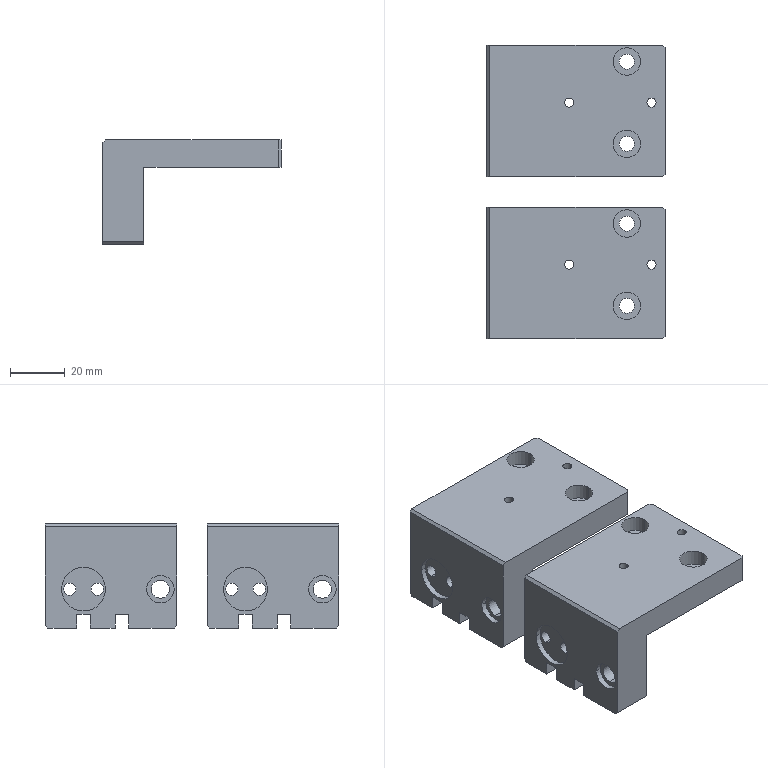NC program | NX | posted with a generic post | part box 65 x 107 x 38 mm
Whole program:
N10 G17 G21 G94 G90
(DRILLING_COPY , TOOL : D6A45)
N12 T01 M6
N14 G54
N16 G17 G0 G90 X-15. Y-4.8 B0. C0. S5000 M3
N18 G43 Z30. H1
N20 G94 G81 G98 Z-1. F350. R3.
N22 X-5.
N24 X18.
N26 G80
N28 G0 X18. Y-4.8 Z30.
N30 M5
(DRILLING_COPY_COPY_COPY_1 , TOOL : 4.5ZT)
N32 T08 M6
N34 G54
N36 G17 G0 G90 X-5. Y-4.8 B0. C0. S2000 M3
N38 G43 Z30. H8
N40 G94 G83 G98 Z-17.352 F300. Q2. R3.
N42 X-15.
N44 G80
N46 G0 X-15. Y-4.8 Z30.
N48 M5
(DRILLING_COPY_COPY_COPY_1_COPY , TOOL : 6.6ZT)
N50 T10 M6
N52 G54
N54 G17 G0 G90 X18. Y-4.8 B0. C0. S2000 M3
N56 G43 Z30. H10
N58 G94 G83 G98 Z-17.983 F300. Q2. R3.
N60 G80
N62 G0 X18. Y-4.8 Z30.
N64 M5
(HOLE_MILLING_COPY , TOOL : D6)
N66 T12 M6
N68 G54
N70 G17 G0 G90 X-10. Y-4.8 B0. C0. S9500 M3
N72 G43 Z30. H12
N74 Z0.5
N76 G94 G3 X-11.225 Y-3.575 R1.225 F1500.
N78 X-12.45 Y-4.8 R1.225
N80 X-12.45 Y-4.8 Z0. I2.45 J0.
N82 X-12.45 Y-4.8 Z-0.5 I2.45 J0.
N84 X-12.45 Y-4.8 Z-1. I2.45 J0.
N86 X-12.45 Y-4.8 Z-1.5 I2.45 J0.
N88 X-12.45 Y-4.8 Z-2. I2.45 J0.
N90 X-10. Y-7.25 R2.45
N92 X-12.45 Y-4.8 R-2.45
N94 X-11.225 Y-6.025 R1.225
N96 X-10. Y-4.8 R1.225
N98 G0 Z0.5
N100 G3 X-12.45 Y-2.35 R2.45
N102 X-14.9 Y-4.8 R2.45
N104 X-14.9 Y-4.8 Z0. I4.9 J0.
N106 X-14.9 Y-4.8 Z-0.5 I4.9 J0.
N108 X-14.9 Y-4.8 Z-1. I4.9 J0.
N110 X-14.9 Y-4.8 Z-1.5 I4.9 J0.
N112 X-14.9 Y-4.8 Z-2. I4.9 J0.
N114 X-10. Y-9.7 R4.9
N116 X-14.9 Y-4.8 R-4.9
N118 X-12.45 Y-7.25 R2.45
N120 X-10. Y-4.8 R2.45
N122 G0 Z30.
N124 X18.
N126 Z0.5
N128 G3 X17.05 Y-3.85 R0.95
N130 X16.1 Y-4.8 R0.95
N132 X16.1 Y-4.8 Z0. I1.9 J0.
N134 X16.1 Y-4.8 Z-0.5 I1.9 J0.
N136 X16.1 Y-4.8 Z-1. I1.9 J0.
N138 X16.1 Y-4.8 Z-1.5 I1.9 J0.
N140 X16.1 Y-4.8 Z-2. I1.9 J0.
N142 X18. Y-6.7 R1.9
N144 X16.1 Y-4.8 R-1.9
N146 X17.05 Y-5.75 R0.95
N148 X18. Y-4.8 R0.95
N150 G0 Z30.
N152 M5
(PLANAR_MILL_COPY_COPY_COPY_COPY_COPY_1 , TOOL : D6A45)
N154 T01 M6
N156 G54
N158 G17 G0 G90 X-11.362 Y-10.541 B0. C0. S9500 M3
N160 G43 Z30. H1
N162 Z0.5
N164 G94 G1 Z-1. F1250.
N166 X-10.866 Y-11.4
N168 G3 X-10. Y-11.9 R1.
N170 X-2.9 Y-4.8 R7.1
N172 X-10. Y-11.9 R-7.1
N174 X-9.134 Y-11.4 R1.
N176 G1 X-8.638 Y-10.541
N178 Z0.5
N180 G0 Z30.
N182 X20.471 Y-6.318
N184 Z0.5
N186 G1 Z-1.
N188 X21.6 Y-5.666
N190 G3 X22.1 Y-4.8 R1.
N192 X18. Y-0.7 R4.1
N194 X22.1 Y-4.8 R-4.1
N196 X21.6 Y-3.934 R1.
N198 G1 X20.471 Y-3.282
N200 Z0.5
N202 G0 Z30.
N204 M5
(刀补 , TOOL : D6)
N206 T12 M6
N208 G54
N210 G17 G0 G90 X-10. Y-4.8 B0. C0. S9500 M3
N212 G43 Z30. H12
N214 Z0.5
N216 G41 G94 G1 X-11.065 Y-3.227 F1500. D12
N218 G3 X-14.95 Y-4.8 R2.261
N220 X-14.95 Y-4.8 Z-1.5 I4.95 J0.
N222 X-10. Y-9.75 Z-2. R4.95
N224 X-5.05 Y-4.8 R4.95
N226 X-10. Y-9.75 R-4.95
N228 X-8.427 Y-5.865 R2.261
N230 G40
N232 G1 X-10. Y-4.8
N234 G0 Z30.
N236 X18.
N238 Z0.5
N240 G41 G1 X18.007 Y-4.7
N242 G3 X16.05 Y-4.8 R0.981
N244 X16.05 Y-4.8 Z-1.5 I1.95 J0.
N246 X18. Y-6.75 Z-2. R1.95
N248 X19.95 Y-4.8 R1.95
N250 X18. Y-6.75 R-1.95
N252 X18.1 Y-4.793 R0.981
N254 G40
N256 G1 X18. Y-4.8
N258 G0 Z30.
N260 M5
N262 M2